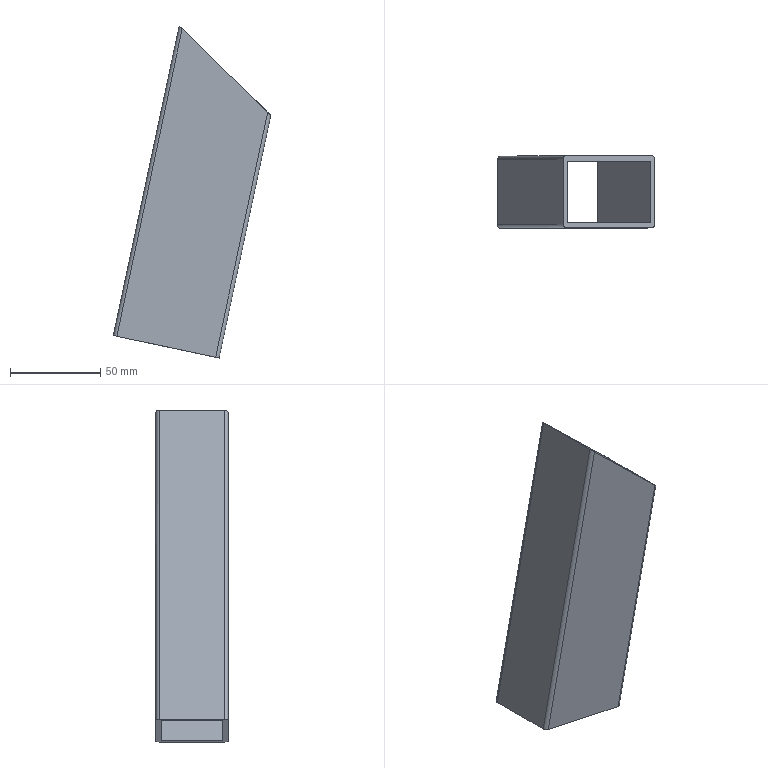Part | STEP file | vertical fixing frame | 1 solid | 14 faces | box 87.186 x 40 x 183.865 mm | volume 87563 mm3 | plane 10 | cylinder 4 | commonest cylinder face diameters 4 x4
STEP:
#1=CARTESIAN_POINT('',(0.,0.,0.));
#2=DIRECTION('',(0.,0.,1.));
#3=DIRECTION('',(1.,0.,0.));
#4=AXIS2_PLACEMENT_3D('',#1,#2,#3);
#5=CARTESIAN_POINT('',(1821.25,153.75,-300.922));
#6=VERTEX_POINT('',#5);
#7=CARTESIAN_POINT('',(1768.509,153.75,-289.712));
#8=VERTEX_POINT('',#7);
#9=CARTESIAN_POINT('',(17.53,153.75,82.471));
#10=DIRECTION('',(-0.9781,0.,0.2079));
#11=VECTOR('',#10,1.);
#12=LINE('',#9,#11);
#13=CARTESIAN_POINT('',(0.,153.75,0.));
#14=DIRECTION('',(0.,-1.,0.));
#15=DIRECTION('',(0.,0.,1.));
#16=AXIS2_PLACEMENT_3D('',#13,#14,#15);
#17=PLANE('',#16);
#18=CARTESIAN_POINT('',(82.471,-17.53));
#19=DIRECTION('',(0.2079,0.9781));
#20=VECTOR('',#19,1.);
#21=LINE('',#18,#20);
#22=(GEOMETRIC_REPRESENTATION_CONTEXT(2)PARAMETRIC_REPRESENTATION_CONTEXT()REPRESENTATION_CONTEXT('',''));
#23=DEFINITIONAL_REPRESENTATION('',(#21),#22);
#24=PCURVE('',#17,#23);
#25=CARTESIAN_POINT('',(1824.185,190.75,-301.546));
#26=DIRECTION('',(0.2079,0.,0.9781));
#27=DIRECTION('',(-0.9781,0.,0.2079));
#28=AXIS2_PLACEMENT_3D('',#25,#26,#27);
#29=PLANE('',#28);
#30=CARTESIAN_POINT('',(1847.017,37.));
#31=DIRECTION('',(1.,0.));
#32=VECTOR('',#31,1.);
#33=LINE('',#30,#32);
#34=(GEOMETRIC_REPRESENTATION_CONTEXT(2)PARAMETRIC_REPRESENTATION_CONTEXT()REPRESENTATION_CONTEXT('',''));
#35=DEFINITIONAL_REPRESENTATION('',(#33),#34);
#36=PCURVE('',#29,#35);
#37=SURFACE_CURVE('',#12,(#24,#36),.PCURVE_S1.);
#38=EDGE_CURVE('',#6,#8,#37,.T.);
#39=ORIENTED_EDGE('',*,*,#38,.T.);
#40=CARTESIAN_POINT('',(1804.549,153.75,-120.155));
#41=VERTEX_POINT('',#40);
#42=CARTESIAN_POINT('',(1768.509,153.75,-289.712));
#43=DIRECTION('',(-0.2079,0.,-0.9781));
#44=VECTOR('',#43,1.);
#45=LINE('',#42,#44);
#46=CARTESIAN_POINT('',(-289.712,-1768.509));
#47=DIRECTION('',(-0.9781,0.2079));
#48=VECTOR('',#47,1.);
#49=LINE('',#46,#48);
#50=(GEOMETRIC_REPRESENTATION_CONTEXT(2)PARAMETRIC_REPRESENTATION_CONTEXT()REPRESENTATION_CONTEXT('',''));
#51=DEFINITIONAL_REPRESENTATION('',(#49),#50);
#52=PCURVE('',#17,#51);
#53=CARTESIAN_POINT('',(1768.509,190.75,-289.712));
#54=DIRECTION('',(0.9781,0.,-0.2079));
#55=DIRECTION('',(0.2079,0.,0.9781));
#56=AXIS2_PLACEMENT_3D('',#53,#54,#55);
#57=PLANE('',#56);
#58=CARTESIAN_POINT('',(0.,37.));
#59=DIRECTION('',(-1.,0.));
#60=VECTOR('',#59,1.);
#61=LINE('',#58,#60);
#62=(GEOMETRIC_REPRESENTATION_CONTEXT(2)PARAMETRIC_REPRESENTATION_CONTEXT()REPRESENTATION_CONTEXT('',''));
#63=DEFINITIONAL_REPRESENTATION('',(#61),#62);
#64=PCURVE('',#57,#63);
#65=SURFACE_CURVE('',#45,(#52,#64),.PCURVE_S1.);
#66=EDGE_CURVE('',#41,#8,#65,.T.);
#67=ORIENTED_EDGE('',*,*,#66,.F.);
#68=CARTESIAN_POINT('',(1850.22,153.75,-164.631));
#69=VERTEX_POINT('',#68);
#70=CARTESIAN_POINT('',(818.299,153.75,840.287));
#71=DIRECTION('',(0.7164,0.,-0.6977));
#72=VECTOR('',#71,1.);
#73=LINE('',#70,#72);
#74=CARTESIAN_POINT('',(840.287,-818.299));
#75=DIRECTION('',(-0.6977,-0.7164));
#76=VECTOR('',#75,1.);
#77=LINE('',#74,#76);
#78=(GEOMETRIC_REPRESENTATION_CONTEXT(2)PARAMETRIC_REPRESENTATION_CONTEXT()REPRESENTATION_CONTEXT('',''));
#79=DEFINITIONAL_REPRESENTATION('',(#77),#78);
#80=PCURVE('',#17,#79);
#81=CARTESIAN_POINT('',(1802.008,190.75,-117.681));
#82=DIRECTION('',(-0.6977,0.,-0.7164));
#83=DIRECTION('',(0.7164,0.,-0.6977));
#84=AXIS2_PLACEMENT_3D('',#81,#82,#83);
#85=PLANE('',#84);
#86=CARTESIAN_POINT('',(-1373.094,37.));
#87=DIRECTION('',(1.,0.));
#88=VECTOR('',#87,1.);
#89=LINE('',#86,#88);
#90=(GEOMETRIC_REPRESENTATION_CONTEXT(2)PARAMETRIC_REPRESENTATION_CONTEXT()REPRESENTATION_CONTEXT('',''));
#91=DEFINITIONAL_REPRESENTATION('',(#89),#90);
#92=PCURVE('',#85,#91);
#93=SURFACE_CURVE('',#73,(#80,#92),.PCURVE_S1.);
#94=EDGE_CURVE('',#41,#69,#93,.T.);
#95=ORIENTED_EDGE('',*,*,#94,.T.);
#96=CARTESIAN_POINT('',(1849.827,153.75,-166.482));
#97=DIRECTION('',(0.2079,0.,0.9781));
#98=VECTOR('',#97,1.);
#99=LINE('',#96,#98);
#100=CARTESIAN_POINT('',(-166.482,-1849.827));
#101=DIRECTION('',(0.9781,-0.2079));
#102=VECTOR('',#101,1.);
#103=LINE('',#100,#102);
#104=(GEOMETRIC_REPRESENTATION_CONTEXT(2)PARAMETRIC_REPRESENTATION_CONTEXT()REPRESENTATION_CONTEXT('',''));
#105=DEFINITIONAL_REPRESENTATION('',(#103),#104);
#106=PCURVE('',#17,#105);
#107=CARTESIAN_POINT('',(1849.827,190.75,-166.482));
#108=DIRECTION('',(-0.9781,0.,0.2079));
#109=DIRECTION('',(-0.2079,0.,-0.9781));
#110=AXIS2_PLACEMENT_3D('',#107,#108,#109);
#111=PLANE('',#110);
#112=CARTESIAN_POINT('',(0.,37.));
#113=DIRECTION('',(-1.,0.));
#114=VECTOR('',#113,1.);
#115=LINE('',#112,#114);
#116=(GEOMETRIC_REPRESENTATION_CONTEXT(2)PARAMETRIC_REPRESENTATION_CONTEXT()REPRESENTATION_CONTEXT('',''));
#117=DEFINITIONAL_REPRESENTATION('',(#115),#116);
#118=PCURVE('',#111,#117);
#119=SURFACE_CURVE('',#99,(#106,#118),.PCURVE_S1.);
#120=EDGE_CURVE('',#6,#69,#119,.T.);
#121=ORIENTED_EDGE('',*,*,#120,.F.);
#122=EDGE_LOOP('',(#39,#67,#95,#121));
#123=FACE_BOUND('',#122,.T.);
#124=ADVANCED_FACE('',(#123),#17,.F.);
#125=CARTESIAN_POINT('',(1804.549,187.75,-120.155));
#126=VERTEX_POINT('',#125);
#127=CARTESIAN_POINT('',(1850.22,187.75,-164.631));
#128=VERTEX_POINT('',#127);
#129=CARTESIAN_POINT('',(818.299,187.75,840.287));
#130=DIRECTION('',(0.7164,0.,-0.6977));
#131=VECTOR('',#130,1.);
#132=LINE('',#129,#131);
#133=CARTESIAN_POINT('',(0.,187.75,0.));
#134=DIRECTION('',(0.,-1.,0.));
#135=DIRECTION('',(0.,0.,1.));
#136=AXIS2_PLACEMENT_3D('',#133,#134,#135);
#137=PLANE('',#136);
#138=CARTESIAN_POINT('',(840.287,-818.299));
#139=DIRECTION('',(-0.6977,-0.7164));
#140=VECTOR('',#139,1.);
#141=LINE('',#138,#140);
#142=(GEOMETRIC_REPRESENTATION_CONTEXT(2)PARAMETRIC_REPRESENTATION_CONTEXT()REPRESENTATION_CONTEXT('',''));
#143=DEFINITIONAL_REPRESENTATION('',(#141),#142);
#144=PCURVE('',#137,#143);
#145=CARTESIAN_POINT('',(-1373.094,3.));
#146=DIRECTION('',(1.,0.));
#147=VECTOR('',#146,1.);
#148=LINE('',#145,#147);
#149=(GEOMETRIC_REPRESENTATION_CONTEXT(2)PARAMETRIC_REPRESENTATION_CONTEXT()REPRESENTATION_CONTEXT('',''));
#150=DEFINITIONAL_REPRESENTATION('',(#148),#149);
#151=PCURVE('',#85,#150);
#152=SURFACE_CURVE('',#132,(#144,#151),.PCURVE_S1.);
#153=EDGE_CURVE('',#126,#128,#152,.T.);
#154=ORIENTED_EDGE('',*,*,#153,.F.);
#155=CARTESIAN_POINT('',(1768.509,187.75,-289.712));
#156=VERTEX_POINT('',#155);
#157=CARTESIAN_POINT('',(1768.509,187.75,-289.712));
#158=DIRECTION('',(-0.2079,0.,-0.9781));
#159=VECTOR('',#158,1.);
#160=LINE('',#157,#159);
#161=CARTESIAN_POINT('',(-289.712,-1768.509));
#162=DIRECTION('',(-0.9781,0.2079));
#163=VECTOR('',#162,1.);
#164=LINE('',#161,#163);
#165=(GEOMETRIC_REPRESENTATION_CONTEXT(2)PARAMETRIC_REPRESENTATION_CONTEXT()REPRESENTATION_CONTEXT('',''));
#166=DEFINITIONAL_REPRESENTATION('',(#164),#165);
#167=PCURVE('',#137,#166);
#168=CARTESIAN_POINT('',(0.,3.));
#169=DIRECTION('',(-1.,0.));
#170=VECTOR('',#169,1.);
#171=LINE('',#168,#170);
#172=(GEOMETRIC_REPRESENTATION_CONTEXT(2)PARAMETRIC_REPRESENTATION_CONTEXT()REPRESENTATION_CONTEXT('',''));
#173=DEFINITIONAL_REPRESENTATION('',(#171),#172);
#174=PCURVE('',#57,#173);
#175=SURFACE_CURVE('',#160,(#167,#174),.PCURVE_S1.);
#176=EDGE_CURVE('',#126,#156,#175,.T.);
#177=ORIENTED_EDGE('',*,*,#176,.T.);
#178=CARTESIAN_POINT('',(1821.25,187.75,-300.922));
#179=VERTEX_POINT('',#178);
#180=CARTESIAN_POINT('',(17.53,187.75,82.471));
#181=DIRECTION('',(-0.9781,0.,0.2079));
#182=VECTOR('',#181,1.);
#183=LINE('',#180,#182);
#184=CARTESIAN_POINT('',(82.471,-17.53));
#185=DIRECTION('',(0.2079,0.9781));
#186=VECTOR('',#185,1.);
#187=LINE('',#184,#186);
#188=(GEOMETRIC_REPRESENTATION_CONTEXT(2)PARAMETRIC_REPRESENTATION_CONTEXT()REPRESENTATION_CONTEXT('',''));
#189=DEFINITIONAL_REPRESENTATION('',(#187),#188);
#190=PCURVE('',#137,#189);
#191=CARTESIAN_POINT('',(1847.017,3.));
#192=DIRECTION('',(1.,0.));
#193=VECTOR('',#192,1.);
#194=LINE('',#191,#193);
#195=(GEOMETRIC_REPRESENTATION_CONTEXT(2)PARAMETRIC_REPRESENTATION_CONTEXT()REPRESENTATION_CONTEXT('',''));
#196=DEFINITIONAL_REPRESENTATION('',(#194),#195);
#197=PCURVE('',#29,#196);
#198=SURFACE_CURVE('',#183,(#190,#197),.PCURVE_S1.);
#199=EDGE_CURVE('',#179,#156,#198,.T.);
#200=ORIENTED_EDGE('',*,*,#199,.F.);
#201=CARTESIAN_POINT('',(1849.827,187.75,-166.482));
#202=DIRECTION('',(0.2079,0.,0.9781));
#203=VECTOR('',#202,1.);
#204=LINE('',#201,#203);
#205=CARTESIAN_POINT('',(-166.482,-1849.827));
#206=DIRECTION('',(0.9781,-0.2079));
#207=VECTOR('',#206,1.);
#208=LINE('',#205,#207);
#209=(GEOMETRIC_REPRESENTATION_CONTEXT(2)PARAMETRIC_REPRESENTATION_CONTEXT()REPRESENTATION_CONTEXT('',''));
#210=DEFINITIONAL_REPRESENTATION('',(#208),#209);
#211=PCURVE('',#137,#210);
#212=CARTESIAN_POINT('',(0.,3.));
#213=DIRECTION('',(-1.,0.));
#214=VECTOR('',#213,1.);
#215=LINE('',#212,#214);
#216=(GEOMETRIC_REPRESENTATION_CONTEXT(2)PARAMETRIC_REPRESENTATION_CONTEXT()REPRESENTATION_CONTEXT('',''));
#217=DEFINITIONAL_REPRESENTATION('',(#215),#216);
#218=PCURVE('',#111,#217);
#219=SURFACE_CURVE('',#204,(#211,#218),.PCURVE_S1.);
#220=EDGE_CURVE('',#179,#128,#219,.T.);
#221=ORIENTED_EDGE('',*,*,#220,.T.);
#222=EDGE_LOOP('',(#154,#177,#200,#221));
#223=FACE_BOUND('',#222,.T.);
#224=ADVANCED_FACE('',(#223),#137,.T.);
#225=CARTESIAN_POINT('',(1821.25,190.75,-300.922));
#226=DIRECTION('',(0.,-1.,0.));
#227=VECTOR('',#226,1.);
#228=LINE('',#225,#227);
#229=CARTESIAN_POINT('',(137.444,0.));
#230=DIRECTION('',(0.,1.));
#231=VECTOR('',#230,1.);
#232=LINE('',#229,#231);
#233=(GEOMETRIC_REPRESENTATION_CONTEXT(2)PARAMETRIC_REPRESENTATION_CONTEXT()REPRESENTATION_CONTEXT('',''));
#234=DEFINITIONAL_REPRESENTATION('',(#232),#233);
#235=PCURVE('',#111,#234);
#236=CARTESIAN_POINT('',(3.,0.));
#237=DIRECTION('',(0.,1.));
#238=VECTOR('',#237,1.);
#239=LINE('',#236,#238);
#240=(GEOMETRIC_REPRESENTATION_CONTEXT(2)PARAMETRIC_REPRESENTATION_CONTEXT()REPRESENTATION_CONTEXT('',''));
#241=DEFINITIONAL_REPRESENTATION('',(#239),#240);
#242=PCURVE('',#29,#241);
#243=SURFACE_CURVE('',#228,(#235,#242),.PCURVE_S1.);
#244=EDGE_CURVE('',#179,#6,#243,.T.);
#245=ORIENTED_EDGE('',*,*,#244,.T.);
#246=ORIENTED_EDGE('',*,*,#120,.T.);
#247=CARTESIAN_POINT('',(1850.22,190.75,-164.631));
#248=DIRECTION('',(0.,-1.,0.));
#249=VECTOR('',#248,1.);
#250=LINE('',#247,#249);
#251=CARTESIAN_POINT('',(-1.892,0.));
#252=DIRECTION('',(0.,1.));
#253=VECTOR('',#252,1.);
#254=LINE('',#251,#253);
#255=(GEOMETRIC_REPRESENTATION_CONTEXT(2)PARAMETRIC_REPRESENTATION_CONTEXT()REPRESENTATION_CONTEXT('',''));
#256=DEFINITIONAL_REPRESENTATION('',(#254),#255);
#257=PCURVE('',#111,#256);
#258=CARTESIAN_POINT('',(67.295,0.));
#259=DIRECTION('',(0.,1.));
#260=VECTOR('',#259,1.);
#261=LINE('',#258,#260);
#262=(GEOMETRIC_REPRESENTATION_CONTEXT(2)PARAMETRIC_REPRESENTATION_CONTEXT()REPRESENTATION_CONTEXT('',''));
#263=DEFINITIONAL_REPRESENTATION('',(#261),#262);
#264=PCURVE('',#85,#263);
#265=SURFACE_CURVE('',#250,(#257,#264),.PCURVE_S1.);
#266=EDGE_CURVE('',#128,#69,#265,.T.);
#267=ORIENTED_EDGE('',*,*,#266,.F.);
#268=ORIENTED_EDGE('',*,*,#220,.F.);
#269=EDGE_LOOP('',(#245,#246,#267,#268));
#270=FACE_BOUND('',#269,.T.);
#271=ADVANCED_FACE('',(#270),#111,.T.);
#272=CARTESIAN_POINT('',(1768.509,190.75,-289.712));
#273=DIRECTION('',(0.,-1.,0.));
#274=VECTOR('',#273,1.);
#275=LINE('',#272,#274);
#276=CARTESIAN_POINT('',(0.,0.));
#277=DIRECTION('',(0.,1.));
#278=VECTOR('',#277,1.);
#279=LINE('',#276,#278);
#280=(GEOMETRIC_REPRESENTATION_CONTEXT(2)PARAMETRIC_REPRESENTATION_CONTEXT()REPRESENTATION_CONTEXT('',''));
#281=DEFINITIONAL_REPRESENTATION('',(#279),#280);
#282=PCURVE('',#57,#281);
#283=CARTESIAN_POINT('',(56.919,0.));
#284=DIRECTION('',(0.,1.));
#285=VECTOR('',#284,1.);
#286=LINE('',#283,#285);
#287=(GEOMETRIC_REPRESENTATION_CONTEXT(2)PARAMETRIC_REPRESENTATION_CONTEXT()REPRESENTATION_CONTEXT('',''));
#288=DEFINITIONAL_REPRESENTATION('',(#286),#287);
#289=PCURVE('',#29,#288);
#290=SURFACE_CURVE('',#275,(#282,#289),.PCURVE_S1.);
#291=EDGE_CURVE('',#156,#8,#290,.T.);
#292=ORIENTED_EDGE('',*,*,#291,.F.);
#293=ORIENTED_EDGE('',*,*,#176,.F.);
#294=CARTESIAN_POINT('',(1804.549,190.75,-120.155));
#295=DIRECTION('',(0.,-1.,0.));
#296=VECTOR('',#295,1.);
#297=LINE('',#294,#296);
#298=CARTESIAN_POINT('',(173.344,0.));
#299=DIRECTION('',(0.,1.));
#300=VECTOR('',#299,1.);
#301=LINE('',#298,#300);
#302=(GEOMETRIC_REPRESENTATION_CONTEXT(2)PARAMETRIC_REPRESENTATION_CONTEXT()REPRESENTATION_CONTEXT('',''));
#303=DEFINITIONAL_REPRESENTATION('',(#301),#302);
#304=PCURVE('',#57,#303);
#305=CARTESIAN_POINT('',(3.547,0.));
#306=DIRECTION('',(0.,1.));
#307=VECTOR('',#306,1.);
#308=LINE('',#305,#307);
#309=(GEOMETRIC_REPRESENTATION_CONTEXT(2)PARAMETRIC_REPRESENTATION_CONTEXT()REPRESENTATION_CONTEXT('',''));
#310=DEFINITIONAL_REPRESENTATION('',(#308),#309);
#311=PCURVE('',#85,#310);
#312=SURFACE_CURVE('',#297,(#304,#311),.PCURVE_S1.);
#313=EDGE_CURVE('',#126,#41,#312,.T.);
#314=ORIENTED_EDGE('',*,*,#313,.T.);
#315=ORIENTED_EDGE('',*,*,#66,.T.);
#316=EDGE_LOOP('',(#292,#293,#314,#315));
#317=FACE_BOUND('',#316,.T.);
#318=ADVANCED_FACE('',(#317),#57,.T.);
#319=CARTESIAN_POINT('',(1765.575,188.75,-289.088));
#320=VERTEX_POINT('',#319);
#321=CARTESIAN_POINT('',(1767.531,190.75,-289.504));
#322=VERTEX_POINT('',#321);
#323=CARTESIAN_POINT('',(1767.531,188.75,-289.504));
#324=DIRECTION('',(-0.2079,0.,-0.9781));
#325=DIRECTION('',(0.9781,0.,-0.2079));
#326=AXIS2_PLACEMENT_3D('',#323,#324,#325);
#327=CIRCLE('',#326,2.);
#328=CARTESIAN_POINT('',(1750.001,188.75,-371.974));
#329=DIRECTION('',(0.2079,0.,0.9781));
#330=DIRECTION('',(-0.9781,0.,0.2079));
#331=AXIS2_PLACEMENT_3D('',#328,#329,#330);
#332=CYLINDRICAL_SURFACE('',#331,2.);
#333=CARTESIAN_POINT('',(9.425,84.313));
#334=DIRECTION('',(-1.,0.));
#335=VECTOR('',#334,1.);
#336=LINE('',#333,#335);
#337=(GEOMETRIC_REPRESENTATION_CONTEXT(2)PARAMETRIC_REPRESENTATION_CONTEXT()REPRESENTATION_CONTEXT('',''));
#338=DEFINITIONAL_REPRESENTATION('',(#336),#337);
#339=PCURVE('',#332,#338);
#340=CARTESIAN_POINT('',(55.919,2.));
#341=CARTESIAN_POINT('',(55.919,5.464));
#342=CARTESIAN_POINT('',(58.919,3.732));
#343=CARTESIAN_POINT('',(61.919,2.));
#344=CARTESIAN_POINT('',(58.919,0.2679));
#345=CARTESIAN_POINT('',(55.919,-1.464));
#346=CARTESIAN_POINT('',(55.919,2.));
#347=(BOUNDED_CURVE()B_SPLINE_CURVE(2,(#340,#341,#342,#343,#344,#345,#346),.UNSPECIFIED.,.T.,.F.)B_SPLINE_CURVE_WITH_KNOTS((1,2,2,2,2,1),(-2.094,0.,2.094,4.189,6.283,8.378),.UNSPECIFIED.)CURVE()GEOMETRIC_REPRESENTATION_ITEM()RATIONAL_B_SPLINE_CURVE((1.,0.5,1.,0.5,1.,0.5,1.))REPRESENTATION_ITEM(''));
#348=(GEOMETRIC_REPRESENTATION_CONTEXT(2)PARAMETRIC_REPRESENTATION_CONTEXT()REPRESENTATION_CONTEXT('',''));
#349=DEFINITIONAL_REPRESENTATION('',(#347),#348);
#350=PCURVE('',#29,#349);
#351=SURFACE_CURVE('',#327,(#339,#350),.PCURVE_S1.);
#352=EDGE_CURVE('',#320,#322,#351,.T.);
#353=ORIENTED_EDGE('',*,*,#352,.F.);
#354=CARTESIAN_POINT('',(1802.008,188.75,-117.681));
#355=VERTEX_POINT('',#354);
#356=CARTESIAN_POINT('',(1765.575,188.75,-289.088));
#357=DIRECTION('',(-0.2079,0.,-0.9781));
#358=VECTOR('',#357,1.);
#359=LINE('',#356,#358);
#360=CARTESIAN_POINT('',(6.283,84.313));
#361=DIRECTION('',(0.,-1.));
#362=VECTOR('',#361,1.);
#363=LINE('',#360,#362);
#364=(GEOMETRIC_REPRESENTATION_CONTEXT(2)PARAMETRIC_REPRESENTATION_CONTEXT()REPRESENTATION_CONTEXT('',''));
#365=DEFINITIONAL_REPRESENTATION('',(#363),#364);
#366=PCURVE('',#332,#365);
#367=CARTESIAN_POINT('',(1765.575,190.75,-289.088));
#368=DIRECTION('',(0.9781,0.,-0.2079));
#369=DIRECTION('',(0.2079,0.,0.9781));
#370=AXIS2_PLACEMENT_3D('',#367,#368,#369);
#371=PLANE('',#370);
#372=CARTESIAN_POINT('',(0.,2.));
#373=DIRECTION('',(-1.,0.));
#374=VECTOR('',#373,1.);
#375=LINE('',#372,#374);
#376=(GEOMETRIC_REPRESENTATION_CONTEXT(2)PARAMETRIC_REPRESENTATION_CONTEXT()REPRESENTATION_CONTEXT('',''));
#377=DEFINITIONAL_REPRESENTATION('',(#375),#376);
#378=PCURVE('',#371,#377);
#379=SURFACE_CURVE('',#359,(#366,#378),.PCURVE_S1.);
#380=EDGE_CURVE('',#355,#320,#379,.T.);
#381=ORIENTED_EDGE('',*,*,#380,.F.);
#382=CARTESIAN_POINT('',(1803.702,190.75,-119.331));
#383=VERTEX_POINT('',#382);
#384=CARTESIAN_POINT('',(1803.702,188.75,-119.331));
#385=DIRECTION('',(0.6977,0.,0.7164));
#386=DIRECTION('',(-0.7164,0.,0.6977));
#387=AXIS2_PLACEMENT_3D('',#384,#385,#386);
#388=ELLIPSE('',#387,2.365,2.);
#389=CARTESIAN_POINT('',(4.712,258.288));
#390=CARTESIAN_POINT('',(4.736,258.318));
#391=CARTESIAN_POINT('',(4.784,258.378));
#392=CARTESIAN_POINT('',(4.855,258.468));
#393=CARTESIAN_POINT('',(4.927,258.556));
#394=CARTESIAN_POINT('',(4.998,258.644));
#395=CARTESIAN_POINT('',(5.069,258.729));
#396=CARTESIAN_POINT('',(5.141,258.812));
#397=CARTESIAN_POINT('',(5.212,258.893));
#398=CARTESIAN_POINT('',(5.284,258.971));
#399=CARTESIAN_POINT('',(5.355,259.045));
#400=CARTESIAN_POINT('',(5.426,259.115));
#401=CARTESIAN_POINT('',(5.498,259.181));
#402=CARTESIAN_POINT('',(5.569,259.242));
#403=CARTESIAN_POINT('',(5.641,259.299));
#404=CARTESIAN_POINT('',(5.712,259.35));
#405=CARTESIAN_POINT('',(5.783,259.396));
#406=CARTESIAN_POINT('',(5.855,259.436));
#407=CARTESIAN_POINT('',(5.926,259.471));
#408=CARTESIAN_POINT('',(5.998,259.499));
#409=CARTESIAN_POINT('',(6.069,259.522));
#410=CARTESIAN_POINT('',(6.14,259.538));
#411=CARTESIAN_POINT('',(6.212,259.547));
#412=CARTESIAN_POINT('',(6.259,259.549));
#413=CARTESIAN_POINT('',(6.283,259.549));
#414=B_SPLINE_CURVE_WITH_KNOTS('',3,(#389,#390,#391,#392,#393,#394,#395,#396,#397,#398,#399,#400,#401,#402,#403,#404,#405,#406,#407,#408,#409,#410,#411,#412,#413),.UNSPECIFIED.,.F.,.F.,(4,1,1,1,1,1,1,1,1,1,1,1,1,1,1,1,1,1,1,1,1,1,4),(4.712,4.784,4.855,4.927,4.998,5.069,5.141,5.212,5.284,5.355,5.426,5.498,5.569,5.641,5.712,5.783,5.855,5.926,5.998,6.069,6.14,6.212,6.283),.QUASI_UNIFORM_KNOTS.);
#415=(GEOMETRIC_REPRESENTATION_CONTEXT(2)PARAMETRIC_REPRESENTATION_CONTEXT()REPRESENTATION_CONTEXT('',''));
#416=DEFINITIONAL_REPRESENTATION('',(#414),#415);
#417=PCURVE('',#332,#416);
#418=CARTESIAN_POINT('',(0.,2.));
#419=CARTESIAN_POINT('',(0.,5.464));
#420=CARTESIAN_POINT('',(3.547,3.732));
#421=CARTESIAN_POINT('',(7.094,2.));
#422=CARTESIAN_POINT('',(3.547,0.2679));
#423=CARTESIAN_POINT('',(0.,-1.464));
#424=CARTESIAN_POINT('',(0.,2.));
#425=(BOUNDED_CURVE()B_SPLINE_CURVE(2,(#418,#419,#420,#421,#422,#423,#424),.UNSPECIFIED.,.T.,.F.)B_SPLINE_CURVE_WITH_KNOTS((1,2,2,2,2,1),(-2.094,0.,2.094,4.189,6.283,8.378),.UNSPECIFIED.)CURVE()GEOMETRIC_REPRESENTATION_ITEM()RATIONAL_B_SPLINE_CURVE((1.,0.5,1.,0.5,1.,0.5,1.))REPRESENTATION_ITEM(''));
#426=(GEOMETRIC_REPRESENTATION_CONTEXT(2)PARAMETRIC_REPRESENTATION_CONTEXT()REPRESENTATION_CONTEXT('',''));
#427=DEFINITIONAL_REPRESENTATION('',(#425),#426);
#428=PCURVE('',#85,#427);
#429=SURFACE_CURVE('',#388,(#417,#428),.PCURVE_S1.);
#430=EDGE_CURVE('',#383,#355,#429,.T.);
#431=ORIENTED_EDGE('',*,*,#430,.F.);
#432=CARTESIAN_POINT('',(1750.001,190.75,-371.974));
#433=DIRECTION('',(0.2079,0.,0.9781));
#434=VECTOR('',#433,1.);
#435=LINE('',#432,#434);
#436=CARTESIAN_POINT('',(4.712,0.));
#437=DIRECTION('',(0.,1.));
#438=VECTOR('',#437,1.);
#439=LINE('',#436,#438);
#440=(GEOMETRIC_REPRESENTATION_CONTEXT(2)PARAMETRIC_REPRESENTATION_CONTEXT()REPRESENTATION_CONTEXT('',''));
#441=DEFINITIONAL_REPRESENTATION('',(#439),#440);
#442=PCURVE('',#332,#441);
#443=CARTESIAN_POINT('',(0.,190.75,0.));
#444=DIRECTION('',(0.,-1.,0.));
#445=DIRECTION('',(0.,0.,1.));
#446=AXIS2_PLACEMENT_3D('',#443,#444,#445);
#447=PLANE('',#446);
#448=CARTESIAN_POINT('',(-371.974,-1750.001));
#449=DIRECTION('',(0.9781,-0.2079));
#450=VECTOR('',#449,1.);
#451=LINE('',#448,#450);
#452=(GEOMETRIC_REPRESENTATION_CONTEXT(2)PARAMETRIC_REPRESENTATION_CONTEXT()REPRESENTATION_CONTEXT('',''));
#453=DEFINITIONAL_REPRESENTATION('',(#451),#452);
#454=PCURVE('',#447,#453);
#455=SURFACE_CURVE('',#435,(#442,#454),.PCURVE_S1.);
#456=EDGE_CURVE('',#322,#383,#455,.T.);
#457=ORIENTED_EDGE('',*,*,#456,.F.);
#458=EDGE_LOOP('',(#353,#381,#431,#457));
#459=FACE_BOUND('',#458,.T.);
#460=ADVANCED_FACE('',(#459),#332,.T.);
#461=CARTESIAN_POINT('',(1767.531,150.75,-289.504));
#462=VERTEX_POINT('',#461);
#463=CARTESIAN_POINT('',(1765.575,152.75,-289.088));
#464=VERTEX_POINT('',#463);
#465=CARTESIAN_POINT('',(1767.531,152.75,-289.504));
#466=DIRECTION('',(-0.2079,0.,-0.9781));
#467=DIRECTION('',(0.9781,0.,-0.2079));
#468=AXIS2_PLACEMENT_3D('',#465,#466,#467);
#469=CIRCLE('',#468,2.);
#470=CARTESIAN_POINT('',(1767.531,152.75,-289.504));
#471=DIRECTION('',(-0.2079,0.,-0.9781));
#472=DIRECTION('',(0.9781,0.,-0.2079));
#473=AXIS2_PLACEMENT_3D('',#470,#471,#472);
#474=CYLINDRICAL_SURFACE('',#473,2.);
#475=CARTESIAN_POINT('',(0.,0.));
#476=DIRECTION('',(1.,0.));
#477=VECTOR('',#476,1.);
#478=LINE('',#475,#477);
#479=(GEOMETRIC_REPRESENTATION_CONTEXT(2)PARAMETRIC_REPRESENTATION_CONTEXT()REPRESENTATION_CONTEXT('',''));
#480=DEFINITIONAL_REPRESENTATION('',(#478),#479);
#481=PCURVE('',#474,#480);
#482=CARTESIAN_POINT('',(55.919,38.));
#483=CARTESIAN_POINT('',(55.919,41.464));
#484=CARTESIAN_POINT('',(58.919,39.732));
#485=CARTESIAN_POINT('',(61.919,38.));
#486=CARTESIAN_POINT('',(58.919,36.268));
#487=CARTESIAN_POINT('',(55.919,34.536));
#488=CARTESIAN_POINT('',(55.919,38.));
#489=(BOUNDED_CURVE()B_SPLINE_CURVE(2,(#482,#483,#484,#485,#486,#487,#488),.UNSPECIFIED.,.T.,.F.)B_SPLINE_CURVE_WITH_KNOTS((1,2,2,2,2,1),(-2.094,0.,2.094,4.189,6.283,8.378),.UNSPECIFIED.)CURVE()GEOMETRIC_REPRESENTATION_ITEM()RATIONAL_B_SPLINE_CURVE((1.,0.5,1.,0.5,1.,0.5,1.))REPRESENTATION_ITEM(''));
#490=(GEOMETRIC_REPRESENTATION_CONTEXT(2)PARAMETRIC_REPRESENTATION_CONTEXT()REPRESENTATION_CONTEXT('',''));
#491=DEFINITIONAL_REPRESENTATION('',(#489),#490);
#492=PCURVE('',#29,#491);
#493=SURFACE_CURVE('',#469,(#481,#492),.PCURVE_S1.);
#494=EDGE_CURVE('',#462,#464,#493,.T.);
#495=ORIENTED_EDGE('',*,*,#494,.F.);
#496=CARTESIAN_POINT('',(1803.702,150.75,-119.331));
#497=VERTEX_POINT('',#496);
#498=CARTESIAN_POINT('',(1767.531,150.75,-289.504));
#499=DIRECTION('',(-0.2079,0.,-0.9781));
#500=VECTOR('',#499,1.);
#501=LINE('',#498,#500);
#502=CARTESIAN_POINT('',(1.571,0.));
#503=DIRECTION('',(0.,1.));
#504=VECTOR('',#503,1.);
#505=LINE('',#502,#504);
#506=(GEOMETRIC_REPRESENTATION_CONTEXT(2)PARAMETRIC_REPRESENTATION_CONTEXT()REPRESENTATION_CONTEXT('',''));
#507=DEFINITIONAL_REPRESENTATION('',(#505),#506);
#508=PCURVE('',#474,#507);
#509=CARTESIAN_POINT('',(0.,150.75,0.));
#510=DIRECTION('',(0.,-1.,0.));
#511=DIRECTION('',(0.,0.,1.));
#512=AXIS2_PLACEMENT_3D('',#509,#510,#511);
#513=PLANE('',#512);
#514=CARTESIAN_POINT('',(-289.504,-1767.531));
#515=DIRECTION('',(-0.9781,0.2079));
#516=VECTOR('',#515,1.);
#517=LINE('',#514,#516);
#518=(GEOMETRIC_REPRESENTATION_CONTEXT(2)PARAMETRIC_REPRESENTATION_CONTEXT()REPRESENTATION_CONTEXT('',''));
#519=DEFINITIONAL_REPRESENTATION('',(#517),#518);
#520=PCURVE('',#513,#519);
#521=SURFACE_CURVE('',#501,(#508,#520),.PCURVE_S1.);
#522=EDGE_CURVE('',#497,#462,#521,.T.);
#523=ORIENTED_EDGE('',*,*,#522,.F.);
#524=CARTESIAN_POINT('',(1802.008,152.75,-117.681));
#525=VERTEX_POINT('',#524);
#526=CARTESIAN_POINT('',(1803.702,152.75,-119.331));
#527=DIRECTION('',(0.6977,0.,0.7164));
#528=DIRECTION('',(0.7164,0.,-0.6977));
#529=AXIS2_PLACEMENT_3D('',#526,#527,#528);
#530=ELLIPSE('',#529,2.365,2.);
#531=CARTESIAN_POINT('',(3.142,-175.236));
#532=CARTESIAN_POINT('',(3.118,-175.236));
#533=CARTESIAN_POINT('',(3.07,-175.234));
#534=CARTESIAN_POINT('',(2.999,-175.225));
#535=CARTESIAN_POINT('',(2.927,-175.209));
#536=CARTESIAN_POINT('',(2.856,-175.186));
#537=CARTESIAN_POINT('',(2.785,-175.158));
#538=CARTESIAN_POINT('',(2.713,-175.123));
#539=CARTESIAN_POINT('',(2.642,-175.083));
#540=CARTESIAN_POINT('',(2.57,-175.037));
#541=CARTESIAN_POINT('',(2.499,-174.986));
#542=CARTESIAN_POINT('',(2.428,-174.929));
#543=CARTESIAN_POINT('',(2.356,-174.868));
#544=CARTESIAN_POINT('',(2.285,-174.802));
#545=CARTESIAN_POINT('',(2.213,-174.731));
#546=CARTESIAN_POINT('',(2.142,-174.657));
#547=CARTESIAN_POINT('',(2.071,-174.58));
#548=CARTESIAN_POINT('',(1.999,-174.499));
#549=CARTESIAN_POINT('',(1.928,-174.416));
#550=CARTESIAN_POINT('',(1.856,-174.331));
#551=CARTESIAN_POINT('',(1.785,-174.243));
#552=CARTESIAN_POINT('',(1.714,-174.155));
#553=CARTESIAN_POINT('',(1.642,-174.065));
#554=CARTESIAN_POINT('',(1.595,-174.005));
#555=CARTESIAN_POINT('',(1.571,-173.975));
#556=B_SPLINE_CURVE_WITH_KNOTS('',3,(#531,#532,#533,#534,#535,#536,#537,#538,#539,#540,#541,#542,#543,#544,#545,#546,#547,#548,#549,#550,#551,#552,#553,#554,#555),.UNSPECIFIED.,.F.,.F.,(4,1,1,1,1,1,1,1,1,1,1,1,1,1,1,1,1,1,1,1,1,1,4),(3.142,3.213,3.284,3.356,3.427,3.499,3.57,3.641,3.713,3.784,3.856,3.927,3.998,4.07,4.141,4.213,4.284,4.355,4.427,4.498,4.57,4.641,4.712),.QUASI_UNIFORM_KNOTS.);
#557=(GEOMETRIC_REPRESENTATION_CONTEXT(2)PARAMETRIC_REPRESENTATION_CONTEXT()REPRESENTATION_CONTEXT('',''));
#558=DEFINITIONAL_REPRESENTATION('',(#556),#557);
#559=PCURVE('',#474,#558);
#560=CARTESIAN_POINT('',(4.729,38.));
#561=CARTESIAN_POINT('',(4.729,34.536));
#562=CARTESIAN_POINT('',(1.182,36.268));
#563=CARTESIAN_POINT('',(-2.365,38.));
#564=CARTESIAN_POINT('',(1.182,39.732));
#565=CARTESIAN_POINT('',(4.729,41.464));
#566=CARTESIAN_POINT('',(4.729,38.));
#567=(BOUNDED_CURVE()B_SPLINE_CURVE(2,(#560,#561,#562,#563,#564,#565,#566),.UNSPECIFIED.,.T.,.F.)B_SPLINE_CURVE_WITH_KNOTS((1,2,2,2,2,1),(-2.094,0.,2.094,4.189,6.283,8.378),.UNSPECIFIED.)CURVE()GEOMETRIC_REPRESENTATION_ITEM()RATIONAL_B_SPLINE_CURVE((1.,0.5,1.,0.5,1.,0.5,1.))REPRESENTATION_ITEM(''));
#568=(GEOMETRIC_REPRESENTATION_CONTEXT(2)PARAMETRIC_REPRESENTATION_CONTEXT()REPRESENTATION_CONTEXT('',''));
#569=DEFINITIONAL_REPRESENTATION('',(#567),#568);
#570=PCURVE('',#85,#569);
#571=SURFACE_CURVE('',#530,(#559,#570),.PCURVE_S1.);
#572=EDGE_CURVE('',#525,#497,#571,.T.);
#573=ORIENTED_EDGE('',*,*,#572,.F.);
#574=CARTESIAN_POINT('',(1802.008,152.75,-117.681));
#575=DIRECTION('',(0.2079,0.,0.9781));
#576=VECTOR('',#575,1.);
#577=LINE('',#574,#576);
#578=CARTESIAN_POINT('',(3.142,-175.236));
#579=DIRECTION('',(0.,-1.));
#580=VECTOR('',#579,1.);
#581=LINE('',#578,#580);
#582=(GEOMETRIC_REPRESENTATION_CONTEXT(2)PARAMETRIC_REPRESENTATION_CONTEXT()REPRESENTATION_CONTEXT('',''));
#583=DEFINITIONAL_REPRESENTATION('',(#581),#582);
#584=PCURVE('',#474,#583);
#585=CARTESIAN_POINT('',(175.236,38.));
#586=DIRECTION('',(1.,0.));
#587=VECTOR('',#586,1.);
#588=LINE('',#585,#587);
#589=(GEOMETRIC_REPRESENTATION_CONTEXT(2)PARAMETRIC_REPRESENTATION_CONTEXT()REPRESENTATION_CONTEXT('',''));
#590=DEFINITIONAL_REPRESENTATION('',(#588),#589);
#591=PCURVE('',#371,#590);
#592=SURFACE_CURVE('',#577,(#584,#591),.PCURVE_S1.);
#593=EDGE_CURVE('',#464,#525,#592,.T.);
#594=ORIENTED_EDGE('',*,*,#593,.F.);
#595=EDGE_LOOP('',(#495,#523,#573,#594));
#596=FACE_BOUND('',#595,.T.);
#597=ADVANCED_FACE('',(#596),#474,.T.);
#598=CARTESIAN_POINT('',(1851.067,150.75,-165.456));
#599=VERTEX_POINT('',#598);
#600=CARTESIAN_POINT('',(1852.761,152.75,-167.105));
#601=VERTEX_POINT('',#600);
#602=CARTESIAN_POINT('',(1851.067,152.75,-165.456));
#603=DIRECTION('',(0.6977,0.,0.7164));
#604=DIRECTION('',(-0.7164,0.,0.6977));
#605=AXIS2_PLACEMENT_3D('',#602,#603,#604);
#606=ELLIPSE('',#605,2.365,2.);
#607=CARTESIAN_POINT('',(1850.805,152.75,-166.69));
#608=DIRECTION('',(0.2079,0.,0.9781));
#609=DIRECTION('',(-0.9781,0.,0.2079));
#610=AXIS2_PLACEMENT_3D('',#607,#608,#609);
#611=CYLINDRICAL_SURFACE('',#610,2.);
#612=CARTESIAN_POINT('',(1.571,1.261));
#613=CARTESIAN_POINT('',(1.595,1.231));
#614=CARTESIAN_POINT('',(1.642,1.171));
#615=CARTESIAN_POINT('',(1.714,1.082));
#616=CARTESIAN_POINT('',(1.785,0.9931));
#617=CARTESIAN_POINT('',(1.856,0.9057));
#618=CARTESIAN_POINT('',(1.928,0.8202));
#619=CARTESIAN_POINT('',(1.999,0.737));
#620=CARTESIAN_POINT('',(2.071,0.6564));
#621=CARTESIAN_POINT('',(2.142,0.5789));
#622=CARTESIAN_POINT('',(2.213,0.5048));
#623=CARTESIAN_POINT('',(2.285,0.4347));
#624=CARTESIAN_POINT('',(2.356,0.3687));
#625=CARTESIAN_POINT('',(2.428,0.3073));
#626=CARTESIAN_POINT('',(2.499,0.2507));
#627=CARTESIAN_POINT('',(2.57,0.1993));
#628=CARTESIAN_POINT('',(2.642,0.1534));
#629=CARTESIAN_POINT('',(2.713,0.113));
#630=CARTESIAN_POINT('',(2.785,0.07853));
#631=CARTESIAN_POINT('',(2.856,0.05007));
#632=CARTESIAN_POINT('',(2.927,0.02778));
#633=CARTESIAN_POINT('',(2.999,0.01178));
#634=CARTESIAN_POINT('',(3.07,0.002146));
#635=CARTESIAN_POINT('',(3.118,-0.00000272));
#636=CARTESIAN_POINT('',(3.142,0.));
#637=B_SPLINE_CURVE_WITH_KNOTS('',3,(#612,#613,#614,#615,#616,#617,#618,#619,#620,#621,#622,#623,#624,#625,#626,#627,#628,#629,#630,#631,#632,#633,#634,#635,#636),.UNSPECIFIED.,.F.,.F.,(4,1,1,1,1,1,1,1,1,1,1,1,1,1,1,1,1,1,1,1,1,1,4),(1.571,1.642,1.714,1.785,1.856,1.928,1.999,2.071,2.142,2.213,2.285,2.356,2.428,2.499,2.57,2.642,2.713,2.785,2.856,2.927,2.999,3.07,3.142),.QUASI_UNIFORM_KNOTS.);
#638=(GEOMETRIC_REPRESENTATION_CONTEXT(2)PARAMETRIC_REPRESENTATION_CONTEXT()REPRESENTATION_CONTEXT('',''));
#639=DEFINITIONAL_REPRESENTATION('',(#637),#638);
#640=PCURVE('',#611,#639);
#641=CARTESIAN_POINT('',(66.113,38.));
#642=CARTESIAN_POINT('',(66.113,41.464));
#643=CARTESIAN_POINT('',(69.66,39.732));
#644=CARTESIAN_POINT('',(73.207,38.));
#645=CARTESIAN_POINT('',(69.66,36.268));
#646=CARTESIAN_POINT('',(66.113,34.536));
#647=CARTESIAN_POINT('',(66.113,38.));
#648=(BOUNDED_CURVE()B_SPLINE_CURVE(2,(#641,#642,#643,#644,#645,#646,#647),.UNSPECIFIED.,.T.,.F.)B_SPLINE_CURVE_WITH_KNOTS((1,2,2,2,2,1),(-2.094,0.,2.094,4.189,6.283,8.378),.UNSPECIFIED.)CURVE()GEOMETRIC_REPRESENTATION_ITEM()RATIONAL_B_SPLINE_CURVE((1.,0.5,1.,0.5,1.,0.5,1.))REPRESENTATION_ITEM(''));
#649=(GEOMETRIC_REPRESENTATION_CONTEXT(2)PARAMETRIC_REPRESENTATION_CONTEXT()REPRESENTATION_CONTEXT('',''));
#650=DEFINITIONAL_REPRESENTATION('',(#648),#649);
#651=PCURVE('',#85,#650);
#652=SURFACE_CURVE('',#606,(#640,#651),.PCURVE_S1.);
#653=EDGE_CURVE('',#599,#601,#652,.T.);
#654=ORIENTED_EDGE('',*,*,#653,.F.);
#655=CARTESIAN_POINT('',(1822.229,150.75,-301.13));
#656=VERTEX_POINT('',#655);
#657=CARTESIAN_POINT('',(1850.805,150.75,-166.69));
#658=DIRECTION('',(0.2079,0.,0.9781));
#659=VECTOR('',#658,1.);
#660=LINE('',#657,#659);
#661=CARTESIAN_POINT('',(1.571,0.));
#662=DIRECTION('',(0.,1.));
#663=VECTOR('',#662,1.);
#664=LINE('',#661,#663);
#665=(GEOMETRIC_REPRESENTATION_CONTEXT(2)PARAMETRIC_REPRESENTATION_CONTEXT()REPRESENTATION_CONTEXT('',''));
#666=DEFINITIONAL_REPRESENTATION('',(#664),#665);
#667=PCURVE('',#611,#666);
#668=CARTESIAN_POINT('',(-166.69,-1850.805));
#669=DIRECTION('',(0.9781,-0.2079));
#670=VECTOR('',#669,1.);
#671=LINE('',#668,#670);
#672=(GEOMETRIC_REPRESENTATION_CONTEXT(2)PARAMETRIC_REPRESENTATION_CONTEXT()REPRESENTATION_CONTEXT('',''));
#673=DEFINITIONAL_REPRESENTATION('',(#671),#672);
#674=PCURVE('',#513,#673);
#675=SURFACE_CURVE('',#660,(#667,#674),.PCURVE_S1.);
#676=EDGE_CURVE('',#656,#599,#675,.T.);
#677=ORIENTED_EDGE('',*,*,#676,.F.);
#678=CARTESIAN_POINT('',(1824.185,152.75,-301.546));
#679=VERTEX_POINT('',#678);
#680=CARTESIAN_POINT('',(1822.229,152.75,-301.13));
#681=DIRECTION('',(-0.2079,0.,-0.9781));
#682=DIRECTION('',(0.9781,0.,-0.2079));
#683=AXIS2_PLACEMENT_3D('',#680,#681,#682);
#684=CIRCLE('',#683,2.);
#685=CARTESIAN_POINT('',(3.142,-137.444));
#686=DIRECTION('',(-1.,0.));
#687=VECTOR('',#686,1.);
#688=LINE('',#685,#687);
#689=(GEOMETRIC_REPRESENTATION_CONTEXT(2)PARAMETRIC_REPRESENTATION_CONTEXT()REPRESENTATION_CONTEXT('',''));
#690=DEFINITIONAL_REPRESENTATION('',(#688),#689);
#691=PCURVE('',#611,#690);
#692=CARTESIAN_POINT('',(0.,38.));
#693=CARTESIAN_POINT('',(0.,41.464));
#694=CARTESIAN_POINT('',(3.,39.732));
#695=CARTESIAN_POINT('',(6.,38.));
#696=CARTESIAN_POINT('',(3.,36.268));
#697=CARTESIAN_POINT('',(0.,34.536));
#698=CARTESIAN_POINT('',(0.,38.));
#699=(BOUNDED_CURVE()B_SPLINE_CURVE(2,(#692,#693,#694,#695,#696,#697,#698),.UNSPECIFIED.,.T.,.F.)B_SPLINE_CURVE_WITH_KNOTS((1,2,2,2,2,1),(-2.094,0.,2.094,4.189,6.283,8.378),.UNSPECIFIED.)CURVE()GEOMETRIC_REPRESENTATION_ITEM()RATIONAL_B_SPLINE_CURVE((1.,0.5,1.,0.5,1.,0.5,1.))REPRESENTATION_ITEM(''));
#700=(GEOMETRIC_REPRESENTATION_CONTEXT(2)PARAMETRIC_REPRESENTATION_CONTEXT()REPRESENTATION_CONTEXT('',''));
#701=DEFINITIONAL_REPRESENTATION('',(#699),#700);
#702=PCURVE('',#29,#701);
#703=SURFACE_CURVE('',#684,(#691,#702),.PCURVE_S1.);
#704=EDGE_CURVE('',#679,#656,#703,.T.);
#705=ORIENTED_EDGE('',*,*,#704,.F.);
#706=CARTESIAN_POINT('',(1824.185,152.75,-301.546));
#707=DIRECTION('',(-0.2079,0.,-0.9781));
#708=VECTOR('',#707,1.);
#709=LINE('',#706,#708);
#710=CARTESIAN_POINT('',(3.142,-137.444));
#711=DIRECTION('',(0.,-1.));
#712=VECTOR('',#711,1.);
#713=LINE('',#710,#712);
#714=(GEOMETRIC_REPRESENTATION_CONTEXT(2)PARAMETRIC_REPRESENTATION_CONTEXT()REPRESENTATION_CONTEXT('',''));
#715=DEFINITIONAL_REPRESENTATION('',(#713),#714);
#716=PCURVE('',#611,#715);
#717=CARTESIAN_POINT('',(1852.761,190.75,-167.105));
#718=DIRECTION('',(-0.9781,0.,0.2079));
#719=DIRECTION('',(-0.2079,0.,-0.9781));
#720=AXIS2_PLACEMENT_3D('',#717,#718,#719);
#721=PLANE('',#720);
#722=CARTESIAN_POINT('',(137.444,38.));
#723=DIRECTION('',(1.,0.));
#724=VECTOR('',#723,1.);
#725=LINE('',#722,#724);
#726=(GEOMETRIC_REPRESENTATION_CONTEXT(2)PARAMETRIC_REPRESENTATION_CONTEXT()REPRESENTATION_CONTEXT('',''));
#727=DEFINITIONAL_REPRESENTATION('',(#725),#726);
#728=PCURVE('',#721,#727);
#729=SURFACE_CURVE('',#709,(#716,#728),.PCURVE_S1.);
#730=EDGE_CURVE('',#601,#679,#729,.T.);
#731=ORIENTED_EDGE('',*,*,#730,.F.);
#732=EDGE_LOOP('',(#654,#677,#705,#731));
#733=FACE_BOUND('',#732,.T.);
#734=ADVANCED_FACE('',(#733),#611,.T.);
#735=CARTESIAN_POINT('',(1852.761,188.75,-167.105));
#736=VERTEX_POINT('',#735);
#737=CARTESIAN_POINT('',(1851.067,190.75,-165.456));
#738=VERTEX_POINT('',#737);
#739=CARTESIAN_POINT('',(1851.067,188.75,-165.456));
#740=DIRECTION('',(0.6977,0.,0.7164));
#741=DIRECTION('',(0.7164,0.,-0.6977));
#742=AXIS2_PLACEMENT_3D('',#739,#740,#741);
#743=ELLIPSE('',#742,2.365,2.);
#744=CARTESIAN_POINT('',(1804.699,188.75,-383.601));
#745=DIRECTION('',(-0.2079,0.,-0.9781));
#746=DIRECTION('',(0.9781,0.,-0.2079));
#747=AXIS2_PLACEMENT_3D('',#744,#745,#746);
#748=CYLINDRICAL_SURFACE('',#747,2.);
#749=CARTESIAN_POINT('',(6.283,-221.757));
#750=CARTESIAN_POINT('',(6.259,-221.757));
#751=CARTESIAN_POINT('',(6.212,-221.759));
#752=CARTESIAN_POINT('',(6.14,-221.769));
#753=CARTESIAN_POINT('',(6.069,-221.785));
#754=CARTESIAN_POINT('',(5.998,-221.807));
#755=CARTESIAN_POINT('',(5.926,-221.836));
#756=CARTESIAN_POINT('',(5.855,-221.87));
#757=CARTESIAN_POINT('',(5.783,-221.91));
#758=CARTESIAN_POINT('',(5.712,-221.956));
#759=CARTESIAN_POINT('',(5.641,-222.008));
#760=CARTESIAN_POINT('',(5.569,-222.064));
#761=CARTESIAN_POINT('',(5.498,-222.126));
#762=CARTESIAN_POINT('',(5.426,-222.192));
#763=CARTESIAN_POINT('',(5.355,-222.262));
#764=CARTESIAN_POINT('',(5.284,-222.336));
#765=CARTESIAN_POINT('',(5.212,-222.413));
#766=CARTESIAN_POINT('',(5.141,-222.494));
#767=CARTESIAN_POINT('',(5.069,-222.577));
#768=CARTESIAN_POINT('',(4.998,-222.663));
#769=CARTESIAN_POINT('',(4.927,-222.75));
#770=CARTESIAN_POINT('',(4.855,-222.839));
#771=CARTESIAN_POINT('',(4.784,-222.928));
#772=CARTESIAN_POINT('',(4.736,-222.988));
#773=CARTESIAN_POINT('',(4.712,-223.018));
#774=B_SPLINE_CURVE_WITH_KNOTS('',3,(#749,#750,#751,#752,#753,#754,#755,#756,#757,#758,#759,#760,#761,#762,#763,#764,#765,#766,#767,#768,#769,#770,#771,#772,#773),.UNSPECIFIED.,.F.,.F.,(4,1,1,1,1,1,1,1,1,1,1,1,1,1,1,1,1,1,1,1,1,1,4),(0.,0.0714,0.1428,0.2142,0.2856,0.357,0.4284,0.4998,0.5712,0.6426,0.714,0.7854,0.8568,0.9282,0.9996,1.071,1.142,1.214,1.285,1.357,1.428,1.499,1.571),.QUASI_UNIFORM_KNOTS.);
#775=(GEOMETRIC_REPRESENTATION_CONTEXT(2)PARAMETRIC_REPRESENTATION_CONTEXT()REPRESENTATION_CONTEXT('',''));
#776=DEFINITIONAL_REPRESENTATION('',(#774),#775);
#777=PCURVE('',#748,#776);
#778=CARTESIAN_POINT('',(70.842,2.));
#779=CARTESIAN_POINT('',(70.842,-1.464));
#780=CARTESIAN_POINT('',(67.295,0.2679));
#781=CARTESIAN_POINT('',(63.748,2.));
#782=CARTESIAN_POINT('',(67.295,3.732));
#783=CARTESIAN_POINT('',(70.842,5.464));
#784=CARTESIAN_POINT('',(70.842,2.));
#785=(BOUNDED_CURVE()B_SPLINE_CURVE(2,(#778,#779,#780,#781,#782,#783,#784),.UNSPECIFIED.,.T.,.F.)B_SPLINE_CURVE_WITH_KNOTS((1,2,2,2,2,1),(-2.094,0.,2.094,4.189,6.283,8.378),.UNSPECIFIED.)CURVE()GEOMETRIC_REPRESENTATION_ITEM()RATIONAL_B_SPLINE_CURVE((1.,0.5,1.,0.5,1.,0.5,1.))REPRESENTATION_ITEM(''));
#786=(GEOMETRIC_REPRESENTATION_CONTEXT(2)PARAMETRIC_REPRESENTATION_CONTEXT()REPRESENTATION_CONTEXT('',''));
#787=DEFINITIONAL_REPRESENTATION('',(#785),#786);
#788=PCURVE('',#85,#787);
#789=SURFACE_CURVE('',#743,(#777,#788),.PCURVE_S1.);
#790=EDGE_CURVE('',#736,#738,#789,.T.);
#791=ORIENTED_EDGE('',*,*,#790,.F.);
#792=CARTESIAN_POINT('',(1824.185,188.75,-301.546));
#793=VERTEX_POINT('',#792);
#794=CARTESIAN_POINT('',(1852.761,188.75,-167.105));
#795=DIRECTION('',(0.2079,0.,0.9781));
#796=VECTOR('',#795,1.);
#797=LINE('',#794,#796);
#798=CARTESIAN_POINT('',(6.283,-221.757));
#799=DIRECTION('',(0.,-1.));
#800=VECTOR('',#799,1.);
#801=LINE('',#798,#800);
#802=(GEOMETRIC_REPRESENTATION_CONTEXT(2)PARAMETRIC_REPRESENTATION_CONTEXT()REPRESENTATION_CONTEXT('',''));
#803=DEFINITIONAL_REPRESENTATION('',(#801),#802);
#804=PCURVE('',#748,#803);
#805=CARTESIAN_POINT('',(0.,2.));
#806=DIRECTION('',(-1.,0.));
#807=VECTOR('',#806,1.);
#808=LINE('',#805,#807);
#809=(GEOMETRIC_REPRESENTATION_CONTEXT(2)PARAMETRIC_REPRESENTATION_CONTEXT()REPRESENTATION_CONTEXT('',''));
#810=DEFINITIONAL_REPRESENTATION('',(#808),#809);
#811=PCURVE('',#721,#810);
#812=SURFACE_CURVE('',#797,(#804,#811),.PCURVE_S1.);
#813=EDGE_CURVE('',#793,#736,#812,.T.);
#814=ORIENTED_EDGE('',*,*,#813,.F.);
#815=CARTESIAN_POINT('',(1822.229,190.75,-301.13));
#816=VERTEX_POINT('',#815);
#817=CARTESIAN_POINT('',(1822.229,188.75,-301.13));
#818=DIRECTION('',(-0.2079,0.,-0.9781));
#819=DIRECTION('',(0.9781,0.,-0.2079));
#820=AXIS2_PLACEMENT_3D('',#817,#818,#819);
#821=CIRCLE('',#820,2.);
#822=CARTESIAN_POINT('',(0.,-84.313));
#823=DIRECTION('',(1.,0.));
#824=VECTOR('',#823,1.);
#825=LINE('',#822,#824);
#826=(GEOMETRIC_REPRESENTATION_CONTEXT(2)PARAMETRIC_REPRESENTATION_CONTEXT()REPRESENTATION_CONTEXT('',''));
#827=DEFINITIONAL_REPRESENTATION('',(#825),#826);
#828=PCURVE('',#748,#827);
#829=CARTESIAN_POINT('',(0.,2.));
#830=CARTESIAN_POINT('',(0.,5.464));
#831=CARTESIAN_POINT('',(3.,3.732));
#832=CARTESIAN_POINT('',(6.,2.));
#833=CARTESIAN_POINT('',(3.,0.2679));
#834=CARTESIAN_POINT('',(0.,-1.464));
#835=CARTESIAN_POINT('',(0.,2.));
#836=(BOUNDED_CURVE()B_SPLINE_CURVE(2,(#829,#830,#831,#832,#833,#834,#835),.UNSPECIFIED.,.T.,.F.)B_SPLINE_CURVE_WITH_KNOTS((1,2,2,2,2,1),(-2.094,0.,2.094,4.189,6.283,8.378),.UNSPECIFIED.)CURVE()GEOMETRIC_REPRESENTATION_ITEM()RATIONAL_B_SPLINE_CURVE((1.,0.5,1.,0.5,1.,0.5,1.))REPRESENTATION_ITEM(''));
#837=(GEOMETRIC_REPRESENTATION_CONTEXT(2)PARAMETRIC_REPRESENTATION_CONTEXT()REPRESENTATION_CONTEXT('',''));
#838=DEFINITIONAL_REPRESENTATION('',(#836),#837);
#839=PCURVE('',#29,#838);
#840=SURFACE_CURVE('',#821,(#828,#839),.PCURVE_S1.);
#841=EDGE_CURVE('',#816,#793,#840,.T.);
#842=ORIENTED_EDGE('',*,*,#841,.F.);
#843=CARTESIAN_POINT('',(1804.699,190.75,-383.601));
#844=DIRECTION('',(-0.2079,0.,-0.9781));
#845=VECTOR('',#844,1.);
#846=LINE('',#843,#845);
#847=CARTESIAN_POINT('',(4.712,0.));
#848=DIRECTION('',(0.,1.));
#849=VECTOR('',#848,1.);
#850=LINE('',#847,#849);
#851=(GEOMETRIC_REPRESENTATION_CONTEXT(2)PARAMETRIC_REPRESENTATION_CONTEXT()REPRESENTATION_CONTEXT('',''));
#852=DEFINITIONAL_REPRESENTATION('',(#850),#851);
#853=PCURVE('',#748,#852);
#854=CARTESIAN_POINT('',(-383.601,-1804.699));
#855=DIRECTION('',(-0.9781,0.2079));
#856=VECTOR('',#855,1.);
#857=LINE('',#854,#856);
#858=(GEOMETRIC_REPRESENTATION_CONTEXT(2)PARAMETRIC_REPRESENTATION_CONTEXT()REPRESENTATION_CONTEXT('',''));
#859=DEFINITIONAL_REPRESENTATION('',(#857),#858);
#860=PCURVE('',#447,#859);
#861=SURFACE_CURVE('',#846,(#853,#860),.PCURVE_S1.);
#862=EDGE_CURVE('',#738,#816,#861,.T.);
#863=ORIENTED_EDGE('',*,*,#862,.F.);
#864=EDGE_LOOP('',(#791,#814,#842,#863));
#865=FACE_BOUND('',#864,.T.);
#866=ADVANCED_FACE('',(#865),#748,.T.);
#867=CARTESIAN_POINT('',(1824.185,150.75,-301.546));
#868=DIRECTION('',(-0.9781,0.,0.2079));
#869=VECTOR('',#868,1.);
#870=LINE('',#867,#869);
#871=CARTESIAN_POINT('',(-301.546,-1824.185));
#872=DIRECTION('',(0.2079,0.9781));
#873=VECTOR('',#872,1.);
#874=LINE('',#871,#873);
#875=(GEOMETRIC_REPRESENTATION_CONTEXT(2)PARAMETRIC_REPRESENTATION_CONTEXT()REPRESENTATION_CONTEXT('',''));
#876=DEFINITIONAL_REPRESENTATION('',(#874),#875);
#877=PCURVE('',#513,#876);
#878=CARTESIAN_POINT('',(0.,40.));
#879=DIRECTION('',(1.,0.));
#880=VECTOR('',#879,1.);
#881=LINE('',#878,#880);
#882=(GEOMETRIC_REPRESENTATION_CONTEXT(2)PARAMETRIC_REPRESENTATION_CONTEXT()REPRESENTATION_CONTEXT('',''));
#883=DEFINITIONAL_REPRESENTATION('',(#881),#882);
#884=PCURVE('',#29,#883);
#885=SURFACE_CURVE('',#870,(#877,#884),.PCURVE_S1.);
#886=EDGE_CURVE('',#656,#462,#885,.T.);
#887=ORIENTED_EDGE('',*,*,#886,.F.);
#888=ORIENTED_EDGE('',*,*,#676,.T.);
#889=CARTESIAN_POINT('',(1802.008,150.75,-117.681));
#890=DIRECTION('',(0.7164,0.,-0.6977));
#891=VECTOR('',#890,1.);
#892=LINE('',#889,#891);
#893=CARTESIAN_POINT('',(-117.681,-1802.008));
#894=DIRECTION('',(-0.6977,-0.7164));
#895=VECTOR('',#894,1.);
#896=LINE('',#893,#895);
#897=(GEOMETRIC_REPRESENTATION_CONTEXT(2)PARAMETRIC_REPRESENTATION_CONTEXT()REPRESENTATION_CONTEXT('',''));
#898=DEFINITIONAL_REPRESENTATION('',(#896),#897);
#899=PCURVE('',#513,#898);
#900=CARTESIAN_POINT('',(0.,40.));
#901=DIRECTION('',(1.,0.));
#902=VECTOR('',#901,1.);
#903=LINE('',#900,#902);
#904=(GEOMETRIC_REPRESENTATION_CONTEXT(2)PARAMETRIC_REPRESENTATION_CONTEXT()REPRESENTATION_CONTEXT('',''));
#905=DEFINITIONAL_REPRESENTATION('',(#903),#904);
#906=PCURVE('',#85,#905);
#907=SURFACE_CURVE('',#892,(#899,#906),.PCURVE_S1.);
#908=EDGE_CURVE('',#497,#599,#907,.T.);
#909=ORIENTED_EDGE('',*,*,#908,.F.);
#910=ORIENTED_EDGE('',*,*,#522,.T.);
#911=EDGE_LOOP('',(#887,#888,#909,#910));
#912=FACE_BOUND('',#911,.T.);
#913=ADVANCED_FACE('',(#912),#513,.T.);
#914=CARTESIAN_POINT('',(1802.008,190.75,-117.681));
#915=DIRECTION('',(0.7164,0.,-0.6977));
#916=VECTOR('',#915,1.);
#917=LINE('',#914,#916);
#918=CARTESIAN_POINT('',(-117.681,-1802.008));
#919=DIRECTION('',(-0.6977,-0.7164));
#920=VECTOR('',#919,1.);
#921=LINE('',#918,#920);
#922=(GEOMETRIC_REPRESENTATION_CONTEXT(2)PARAMETRIC_REPRESENTATION_CONTEXT()REPRESENTATION_CONTEXT('',''));
#923=DEFINITIONAL_REPRESENTATION('',(#921),#922);
#924=PCURVE('',#447,#923);
#925=CARTESIAN_POINT('',(0.,0.));
#926=DIRECTION('',(1.,0.));
#927=VECTOR('',#926,1.);
#928=LINE('',#925,#927);
#929=(GEOMETRIC_REPRESENTATION_CONTEXT(2)PARAMETRIC_REPRESENTATION_CONTEXT()REPRESENTATION_CONTEXT('',''));
#930=DEFINITIONAL_REPRESENTATION('',(#928),#929);
#931=PCURVE('',#85,#930);
#932=SURFACE_CURVE('',#917,(#924,#931),.PCURVE_S1.);
#933=EDGE_CURVE('',#383,#738,#932,.T.);
#934=ORIENTED_EDGE('',*,*,#933,.T.);
#935=ORIENTED_EDGE('',*,*,#862,.T.);
#936=CARTESIAN_POINT('',(1824.185,190.75,-301.546));
#937=DIRECTION('',(-0.9781,0.,0.2079));
#938=VECTOR('',#937,1.);
#939=LINE('',#936,#938);
#940=CARTESIAN_POINT('',(-301.546,-1824.185));
#941=DIRECTION('',(0.2079,0.9781));
#942=VECTOR('',#941,1.);
#943=LINE('',#940,#942);
#944=(GEOMETRIC_REPRESENTATION_CONTEXT(2)PARAMETRIC_REPRESENTATION_CONTEXT()REPRESENTATION_CONTEXT('',''));
#945=DEFINITIONAL_REPRESENTATION('',(#943),#944);
#946=PCURVE('',#447,#945);
#947=CARTESIAN_POINT('',(0.,0.));
#948=DIRECTION('',(1.,0.));
#949=VECTOR('',#948,1.);
#950=LINE('',#947,#949);
#951=(GEOMETRIC_REPRESENTATION_CONTEXT(2)PARAMETRIC_REPRESENTATION_CONTEXT()REPRESENTATION_CONTEXT('',''));
#952=DEFINITIONAL_REPRESENTATION('',(#950),#951);
#953=PCURVE('',#29,#952);
#954=SURFACE_CURVE('',#939,(#946,#953),.PCURVE_S1.);
#955=EDGE_CURVE('',#816,#322,#954,.T.);
#956=ORIENTED_EDGE('',*,*,#955,.T.);
#957=ORIENTED_EDGE('',*,*,#456,.T.);
#958=EDGE_LOOP('',(#934,#935,#956,#957));
#959=FACE_BOUND('',#958,.T.);
#960=ADVANCED_FACE('',(#959),#447,.F.);
#961=ORIENTED_EDGE('',*,*,#955,.F.);
#962=ORIENTED_EDGE('',*,*,#841,.T.);
#963=CARTESIAN_POINT('',(1824.185,190.75,-301.546));
#964=DIRECTION('',(0.,-1.,0.));
#965=VECTOR('',#964,1.);
#966=LINE('',#963,#965);
#967=CARTESIAN_POINT('',(0.,0.));
#968=DIRECTION('',(0.,1.));
#969=VECTOR('',#968,1.);
#970=LINE('',#967,#969);
#971=(GEOMETRIC_REPRESENTATION_CONTEXT(2)PARAMETRIC_REPRESENTATION_CONTEXT()REPRESENTATION_CONTEXT('',''));
#972=DEFINITIONAL_REPRESENTATION('',(#970),#971);
#973=PCURVE('',#29,#972);
#974=CARTESIAN_POINT('',(137.444,0.));
#975=DIRECTION('',(0.,1.));
#976=VECTOR('',#975,1.);
#977=LINE('',#974,#976);
#978=(GEOMETRIC_REPRESENTATION_CONTEXT(2)PARAMETRIC_REPRESENTATION_CONTEXT()REPRESENTATION_CONTEXT('',''));
#979=DEFINITIONAL_REPRESENTATION('',(#977),#978);
#980=PCURVE('',#721,#979);
#981=SURFACE_CURVE('',#966,(#973,#980),.PCURVE_S1.);
#982=EDGE_CURVE('',#793,#679,#981,.T.);
#983=ORIENTED_EDGE('',*,*,#982,.T.);
#984=ORIENTED_EDGE('',*,*,#704,.T.);
#985=ORIENTED_EDGE('',*,*,#886,.T.);
#986=ORIENTED_EDGE('',*,*,#494,.T.);
#987=CARTESIAN_POINT('',(1765.575,190.75,-289.088));
#988=DIRECTION('',(0.,-1.,0.));
#989=VECTOR('',#988,1.);
#990=LINE('',#987,#989);
#991=CARTESIAN_POINT('',(59.919,0.));
#992=DIRECTION('',(0.,1.));
#993=VECTOR('',#992,1.);
#994=LINE('',#991,#993);
#995=(GEOMETRIC_REPRESENTATION_CONTEXT(2)PARAMETRIC_REPRESENTATION_CONTEXT()REPRESENTATION_CONTEXT('',''));
#996=DEFINITIONAL_REPRESENTATION('',(#994),#995);
#997=PCURVE('',#29,#996);
#998=CARTESIAN_POINT('',(0.,0.));
#999=DIRECTION('',(0.,1.));
#1000=VECTOR('',#999,1.);
#1001=LINE('',#998,#1000);
#1002=(GEOMETRIC_REPRESENTATION_CONTEXT(2)PARAMETRIC_REPRESENTATION_CONTEXT()REPRESENTATION_CONTEXT('',''));
#1003=DEFINITIONAL_REPRESENTATION('',(#1001),#1002);
#1004=PCURVE('',#371,#1003);
#1005=SURFACE_CURVE('',#990,(#997,#1004),.PCURVE_S1.);
#1006=EDGE_CURVE('',#320,#464,#1005,.T.);
#1007=ORIENTED_EDGE('',*,*,#1006,.F.);
#1008=ORIENTED_EDGE('',*,*,#352,.T.);
#1009=EDGE_LOOP('',(#961,#962,#983,#984,#985,#986,#1007,#1008));
#1010=FACE_BOUND('',#1009,.T.);
#1011=ORIENTED_EDGE('',*,*,#244,.F.);
#1012=ORIENTED_EDGE('',*,*,#199,.T.);
#1013=ORIENTED_EDGE('',*,*,#291,.T.);
#1014=ORIENTED_EDGE('',*,*,#38,.F.);
#1015=EDGE_LOOP('',(#1011,#1012,#1013,#1014));
#1016=FACE_BOUND('',#1015,.T.);
#1017=ADVANCED_FACE('',(#1010,#1016),#29,.F.);
#1018=ORIENTED_EDGE('',*,*,#982,.F.);
#1019=ORIENTED_EDGE('',*,*,#813,.T.);
#1020=CARTESIAN_POINT('',(1852.761,190.75,-167.105));
#1021=DIRECTION('',(0.,-1.,0.));
#1022=VECTOR('',#1021,1.);
#1023=LINE('',#1020,#1022);
#1024=CARTESIAN_POINT('',(0.,0.));
#1025=DIRECTION('',(0.,1.));
#1026=VECTOR('',#1025,1.);
#1027=LINE('',#1024,#1026);
#1028=(GEOMETRIC_REPRESENTATION_CONTEXT(2)PARAMETRIC_REPRESENTATION_CONTEXT()REPRESENTATION_CONTEXT('',''));
#1029=DEFINITIONAL_REPRESENTATION('',(#1027),#1028);
#1030=PCURVE('',#721,#1029);
#1031=CARTESIAN_POINT('',(70.842,0.));
#1032=DIRECTION('',(0.,1.));
#1033=VECTOR('',#1032,1.);
#1034=LINE('',#1031,#1033);
#1035=(GEOMETRIC_REPRESENTATION_CONTEXT(2)PARAMETRIC_REPRESENTATION_CONTEXT()REPRESENTATION_CONTEXT('',''));
#1036=DEFINITIONAL_REPRESENTATION('',(#1034),#1035);
#1037=PCURVE('',#85,#1036);
#1038=SURFACE_CURVE('',#1023,(#1030,#1037),.PCURVE_S1.);
#1039=EDGE_CURVE('',#736,#601,#1038,.T.);
#1040=ORIENTED_EDGE('',*,*,#1039,.T.);
#1041=ORIENTED_EDGE('',*,*,#730,.T.);
#1042=EDGE_LOOP('',(#1018,#1019,#1040,#1041));
#1043=FACE_BOUND('',#1042,.T.);
#1044=ADVANCED_FACE('',(#1043),#721,.F.);
#1045=ORIENTED_EDGE('',*,*,#1039,.F.);
#1046=ORIENTED_EDGE('',*,*,#790,.T.);
#1047=ORIENTED_EDGE('',*,*,#933,.F.);
#1048=ORIENTED_EDGE('',*,*,#430,.T.);
#1049=CARTESIAN_POINT('',(1802.008,190.75,-117.681));
#1050=DIRECTION('',(0.,-1.,0.));
#1051=VECTOR('',#1050,1.);
#1052=LINE('',#1049,#1051);
#1053=CARTESIAN_POINT('',(0.,0.));
#1054=DIRECTION('',(0.,1.));
#1055=VECTOR('',#1054,1.);
#1056=LINE('',#1053,#1055);
#1057=(GEOMETRIC_REPRESENTATION_CONTEXT(2)PARAMETRIC_REPRESENTATION_CONTEXT()REPRESENTATION_CONTEXT('',''));
#1058=DEFINITIONAL_REPRESENTATION('',(#1056),#1057);
#1059=PCURVE('',#85,#1058);
#1060=CARTESIAN_POINT('',(175.236,0.));
#1061=DIRECTION('',(0.,1.));
#1062=VECTOR('',#1061,1.);
#1063=LINE('',#1060,#1062);
#1064=(GEOMETRIC_REPRESENTATION_CONTEXT(2)PARAMETRIC_REPRESENTATION_CONTEXT()REPRESENTATION_CONTEXT('',''));
#1065=DEFINITIONAL_REPRESENTATION('',(#1063),#1064);
#1066=PCURVE('',#371,#1065);
#1067=SURFACE_CURVE('',#1052,(#1059,#1066),.PCURVE_S1.);
#1068=EDGE_CURVE('',#355,#525,#1067,.T.);
#1069=ORIENTED_EDGE('',*,*,#1068,.T.);
#1070=ORIENTED_EDGE('',*,*,#572,.T.);
#1071=ORIENTED_EDGE('',*,*,#908,.T.);
#1072=ORIENTED_EDGE('',*,*,#653,.T.);
#1073=EDGE_LOOP('',(#1045,#1046,#1047,#1048,#1069,#1070,#1071,#1072));
#1074=FACE_BOUND('',#1073,.T.);
#1075=ORIENTED_EDGE('',*,*,#153,.T.);
#1076=ORIENTED_EDGE('',*,*,#266,.T.);
#1077=ORIENTED_EDGE('',*,*,#94,.F.);
#1078=ORIENTED_EDGE('',*,*,#313,.F.);
#1079=EDGE_LOOP('',(#1075,#1076,#1077,#1078));
#1080=FACE_BOUND('',#1079,.T.);
#1081=ADVANCED_FACE('',(#1074,#1080),#85,.F.);
#1082=ORIENTED_EDGE('',*,*,#1006,.T.);
#1083=ORIENTED_EDGE('',*,*,#593,.T.);
#1084=ORIENTED_EDGE('',*,*,#1068,.F.);
#1085=ORIENTED_EDGE('',*,*,#380,.T.);
#1086=EDGE_LOOP('',(#1082,#1083,#1084,#1085));
#1087=FACE_BOUND('',#1086,.T.);
#1088=ADVANCED_FACE('',(#1087),#371,.F.);
#1089=CLOSED_SHELL('',(#124,#224,#271,#318,#460,#597,#734,#866,#913,#960,#1017,#1044,#1081,#1088));
#1090=MANIFOLD_SOLID_BREP('',#1089);
#1091=(LENGTH_UNIT()NAMED_UNIT(*)SI_UNIT(.MILLI.,.METRE.));
#1092=UNCERTAINTY_MEASURE_WITH_UNIT(LENGTH_MEASURE(0.0000001),#1091,'','');
#1093=(NAMED_UNIT(*)PLANE_ANGLE_UNIT()SI_UNIT($,.RADIAN.));
#1094=(NAMED_UNIT(*)SI_UNIT($,.STERADIAN.)SOLID_ANGLE_UNIT());
#1095=(GEOMETRIC_REPRESENTATION_CONTEXT(3)GLOBAL_UNCERTAINTY_ASSIGNED_CONTEXT((#1092))GLOBAL_UNIT_ASSIGNED_CONTEXT((#1091,#1093,#1094))REPRESENTATION_CONTEXT('',''));
#1096=ADVANCED_BREP_SHAPE_REPRESENTATION('',(#4,#1090),#1095);